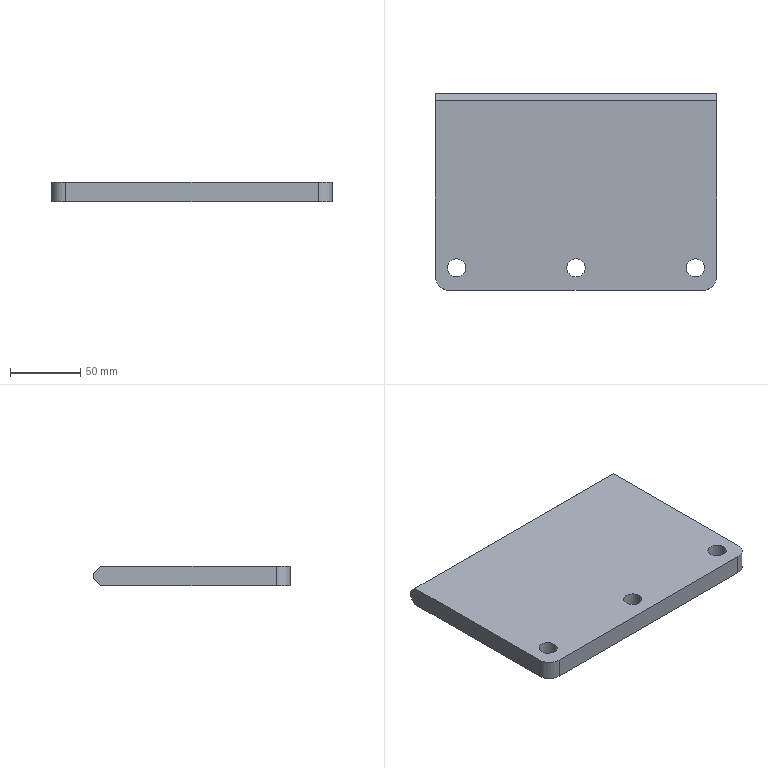Part | SolidWorks | features ICE 2, Chamfer 1, Extrusion 1, Fillet 1 | 1 solid | 16 faces | box 200 x 140 x 14 mm | volume 380824 mm3 | cylinder 8 | plane 8 | commonest cylinder face diameters 13 x6 20 x2
STEP:
#1=CARTESIAN_POINT('',(191.5,16.,14.));
#2=VERTEX_POINT('',#1);
#3=CARTESIAN_POINT('',(178.5,16.,14.));
#4=VERTEX_POINT('',#3);
#5=CARTESIAN_POINT('',(185.,16.,14.));
#6=DIRECTION('',(0.,0.,-1.));
#7=DIRECTION('',(-1.,0.,0.));
#8=AXIS2_PLACEMENT_3D('',#5,#6,#7);
#9=CIRCLE('',#8,6.5);
#10=EDGE_CURVE('',#2,#4,#9,.T.);
#11=ORIENTED_EDGE('',*,*,#10,.F.);
#12=CARTESIAN_POINT('',(191.5,16.,0.));
#13=VERTEX_POINT('',#12);
#14=CARTESIAN_POINT('',(191.5,16.,14.));
#15=DIRECTION('',(0.,0.,-1.));
#16=VECTOR('',#15,1000.);
#17=LINE('',#14,#16);
#18=EDGE_CURVE('',#2,#13,#17,.T.);
#19=ORIENTED_EDGE('',*,*,#18,.T.);
#20=CARTESIAN_POINT('',(178.5,16.,0.));
#21=VERTEX_POINT('',#20);
#22=CARTESIAN_POINT('',(185.,16.,0.));
#23=DIRECTION('',(0.,0.,-1.));
#24=DIRECTION('',(-1.,0.,0.));
#25=AXIS2_PLACEMENT_3D('',#22,#23,#24);
#26=CIRCLE('',#25,6.5);
#27=EDGE_CURVE('',#13,#21,#26,.T.);
#28=ORIENTED_EDGE('',*,*,#27,.T.);
#29=CARTESIAN_POINT('',(178.5,16.,14.));
#30=DIRECTION('',(0.,0.,-1.));
#31=VECTOR('',#30,1000.);
#32=LINE('',#29,#31);
#33=EDGE_CURVE('',#4,#21,#32,.T.);
#34=ORIENTED_EDGE('',*,*,#33,.F.);
#35=EDGE_LOOP('',(#11,#19,#28,#34));
#36=FACE_OUTER_BOUND('',#35,.T.);
#37=CARTESIAN_POINT('',(185.,16.,14.));
#38=DIRECTION('',(0.,0.,-1.));
#39=DIRECTION('',(-1.,0.,0.));
#40=AXIS2_PLACEMENT_3D('',#37,#38,#39);
#41=CYLINDRICAL_SURFACE('',#40,6.5);
#42=ADVANCED_FACE('',(#36),#41,.F.);
#43=CARTESIAN_POINT('',(106.5,16.,14.));
#44=VERTEX_POINT('',#43);
#45=CARTESIAN_POINT('',(93.5,16.,14.));
#46=VERTEX_POINT('',#45);
#47=CARTESIAN_POINT('',(100.,16.,14.));
#48=DIRECTION('',(0.,0.,-1.));
#49=DIRECTION('',(-1.,0.,0.));
#50=AXIS2_PLACEMENT_3D('',#47,#48,#49);
#51=CIRCLE('',#50,6.5);
#52=EDGE_CURVE('',#44,#46,#51,.T.);
#53=ORIENTED_EDGE('',*,*,#52,.F.);
#54=CARTESIAN_POINT('',(106.5,16.,0.));
#55=VERTEX_POINT('',#54);
#56=CARTESIAN_POINT('',(106.5,16.,14.));
#57=DIRECTION('',(0.,0.,-1.));
#58=VECTOR('',#57,1000.);
#59=LINE('',#56,#58);
#60=EDGE_CURVE('',#44,#55,#59,.T.);
#61=ORIENTED_EDGE('',*,*,#60,.T.);
#62=CARTESIAN_POINT('',(93.5,16.,0.));
#63=VERTEX_POINT('',#62);
#64=CARTESIAN_POINT('',(100.,16.,0.));
#65=DIRECTION('',(0.,0.,-1.));
#66=DIRECTION('',(-1.,0.,0.));
#67=AXIS2_PLACEMENT_3D('',#64,#65,#66);
#68=CIRCLE('',#67,6.5);
#69=EDGE_CURVE('',#55,#63,#68,.T.);
#70=ORIENTED_EDGE('',*,*,#69,.T.);
#71=CARTESIAN_POINT('',(93.5,16.,14.));
#72=DIRECTION('',(0.,0.,-1.));
#73=VECTOR('',#72,1000.);
#74=LINE('',#71,#73);
#75=EDGE_CURVE('',#46,#63,#74,.T.);
#76=ORIENTED_EDGE('',*,*,#75,.F.);
#77=EDGE_LOOP('',(#53,#61,#70,#76));
#78=FACE_OUTER_BOUND('',#77,.T.);
#79=CARTESIAN_POINT('',(100.,16.,14.));
#80=DIRECTION('',(0.,0.,-1.));
#81=DIRECTION('',(-1.,0.,0.));
#82=AXIS2_PLACEMENT_3D('',#79,#80,#81);
#83=CYLINDRICAL_SURFACE('',#82,6.5);
#84=ADVANCED_FACE('',(#78),#83,.F.);
#85=CARTESIAN_POINT('',(21.5,16.,14.));
#86=VERTEX_POINT('',#85);
#87=CARTESIAN_POINT('',(8.5,16.,14.));
#88=VERTEX_POINT('',#87);
#89=CARTESIAN_POINT('',(15.,16.,14.));
#90=DIRECTION('',(0.,0.,-1.));
#91=DIRECTION('',(-1.,0.,0.));
#92=AXIS2_PLACEMENT_3D('',#89,#90,#91);
#93=CIRCLE('',#92,6.5);
#94=EDGE_CURVE('',#86,#88,#93,.T.);
#95=ORIENTED_EDGE('',*,*,#94,.F.);
#96=CARTESIAN_POINT('',(21.5,16.,0.));
#97=VERTEX_POINT('',#96);
#98=CARTESIAN_POINT('',(21.5,16.,14.));
#99=DIRECTION('',(0.,0.,-1.));
#100=VECTOR('',#99,1000.);
#101=LINE('',#98,#100);
#102=EDGE_CURVE('',#86,#97,#101,.T.);
#103=ORIENTED_EDGE('',*,*,#102,.T.);
#104=CARTESIAN_POINT('',(8.5,16.,0.));
#105=VERTEX_POINT('',#104);
#106=CARTESIAN_POINT('',(15.,16.,0.));
#107=DIRECTION('',(0.,0.,-1.));
#108=DIRECTION('',(-1.,0.,0.));
#109=AXIS2_PLACEMENT_3D('',#106,#107,#108);
#110=CIRCLE('',#109,6.5);
#111=EDGE_CURVE('',#97,#105,#110,.T.);
#112=ORIENTED_EDGE('',*,*,#111,.T.);
#113=CARTESIAN_POINT('',(8.5,16.,14.));
#114=DIRECTION('',(0.,0.,-1.));
#115=VECTOR('',#114,1000.);
#116=LINE('',#113,#115);
#117=EDGE_CURVE('',#88,#105,#116,.T.);
#118=ORIENTED_EDGE('',*,*,#117,.F.);
#119=EDGE_LOOP('',(#95,#103,#112,#118));
#120=FACE_OUTER_BOUND('',#119,.T.);
#121=CARTESIAN_POINT('',(15.,16.,14.));
#122=DIRECTION('',(0.,0.,-1.));
#123=DIRECTION('',(-1.,0.,0.));
#124=AXIS2_PLACEMENT_3D('',#121,#122,#123);
#125=CYLINDRICAL_SURFACE('',#124,6.5);
#126=ADVANCED_FACE('',(#120),#125,.F.);
#127=CARTESIAN_POINT('',(0.,135.,0.));
#128=VERTEX_POINT('',#127);
#129=CARTESIAN_POINT('',(0.,10.,0.));
#130=VERTEX_POINT('',#129);
#131=CARTESIAN_POINT('',(0.,0.,0.));
#132=DIRECTION('',(0.,-1.,0.));
#133=VECTOR('',#132,1000.);
#134=LINE('',#131,#133);
#135=EDGE_CURVE('',#128,#130,#134,.T.);
#136=ORIENTED_EDGE('',*,*,#135,.T.);
#137=CARTESIAN_POINT('',(0.,10.,14.));
#138=VERTEX_POINT('',#137);
#139=CARTESIAN_POINT('',(0.,10.,14.));
#140=DIRECTION('',(0.,0.,1.));
#141=VECTOR('',#140,1000.);
#142=LINE('',#139,#141);
#143=EDGE_CURVE('',#130,#138,#142,.T.);
#144=ORIENTED_EDGE('',*,*,#143,.T.);
#145=CARTESIAN_POINT('',(0.,135.,14.));
#146=VERTEX_POINT('',#145);
#147=CARTESIAN_POINT('',(0.,0.,14.));
#148=DIRECTION('',(0.,-1.,0.));
#149=VECTOR('',#148,1000.);
#150=LINE('',#147,#149);
#151=EDGE_CURVE('',#146,#138,#150,.T.);
#152=ORIENTED_EDGE('',*,*,#151,.F.);
#153=CARTESIAN_POINT('',(0.,140.,9.));
#154=VERTEX_POINT('',#153);
#155=CARTESIAN_POINT('',(0.,135.,14.));
#156=DIRECTION('',(0.,0.7071,-0.7071));
#157=VECTOR('',#156,1000.);
#158=LINE('',#155,#157);
#159=EDGE_CURVE('',#146,#154,#158,.T.);
#160=ORIENTED_EDGE('',*,*,#159,.T.);
#161=CARTESIAN_POINT('',(0.,140.,5.));
#162=VERTEX_POINT('',#161);
#163=CARTESIAN_POINT('',(0.,140.,14.));
#164=DIRECTION('',(0.,0.,-1.));
#165=VECTOR('',#164,1000.);
#166=LINE('',#163,#165);
#167=EDGE_CURVE('',#154,#162,#166,.T.);
#168=ORIENTED_EDGE('',*,*,#167,.T.);
#169=CARTESIAN_POINT('',(0.,140.,5.));
#170=DIRECTION('',(0.,-0.7071,-0.7071));
#171=VECTOR('',#170,1000.);
#172=LINE('',#169,#171);
#173=EDGE_CURVE('',#162,#128,#172,.T.);
#174=ORIENTED_EDGE('',*,*,#173,.T.);
#175=EDGE_LOOP('',(#136,#144,#152,#160,#168,#174));
#176=FACE_OUTER_BOUND('',#175,.T.);
#177=CARTESIAN_POINT('',(0.,0.,14.));
#178=DIRECTION('',(1.,0.,0.));
#179=DIRECTION('',(0.,0.,-1.));
#180=AXIS2_PLACEMENT_3D('',#177,#178,#179);
#181=PLANE('',#180);
#182=ADVANCED_FACE('',(#176),#181,.F.);
#183=CARTESIAN_POINT('',(10.,0.,0.));
#184=VERTEX_POINT('',#183);
#185=CARTESIAN_POINT('',(190.,0.,0.));
#186=VERTEX_POINT('',#185);
#187=CARTESIAN_POINT('',(0.,0.,0.));
#188=DIRECTION('',(1.,0.,0.));
#189=VECTOR('',#188,1000.);
#190=LINE('',#187,#189);
#191=EDGE_CURVE('',#184,#186,#190,.T.);
#192=ORIENTED_EDGE('',*,*,#191,.T.);
#193=CARTESIAN_POINT('',(190.,0.,14.));
#194=VERTEX_POINT('',#193);
#195=CARTESIAN_POINT('',(190.,0.,14.));
#196=DIRECTION('',(0.,0.,1.));
#197=VECTOR('',#196,1000.);
#198=LINE('',#195,#197);
#199=EDGE_CURVE('',#186,#194,#198,.T.);
#200=ORIENTED_EDGE('',*,*,#199,.T.);
#201=CARTESIAN_POINT('',(10.,0.,14.));
#202=VERTEX_POINT('',#201);
#203=CARTESIAN_POINT('',(0.,0.,14.));
#204=DIRECTION('',(1.,0.,0.));
#205=VECTOR('',#204,1000.);
#206=LINE('',#203,#205);
#207=EDGE_CURVE('',#202,#194,#206,.T.);
#208=ORIENTED_EDGE('',*,*,#207,.F.);
#209=CARTESIAN_POINT('',(10.,0.,14.));
#210=DIRECTION('',(0.,0.,-1.));
#211=VECTOR('',#210,1000.);
#212=LINE('',#209,#211);
#213=EDGE_CURVE('',#202,#184,#212,.T.);
#214=ORIENTED_EDGE('',*,*,#213,.T.);
#215=EDGE_LOOP('',(#192,#200,#208,#214));
#216=FACE_OUTER_BOUND('',#215,.T.);
#217=CARTESIAN_POINT('',(0.,0.,14.));
#218=DIRECTION('',(0.,1.,0.));
#219=DIRECTION('',(0.,0.,1.));
#220=AXIS2_PLACEMENT_3D('',#217,#218,#219);
#221=PLANE('',#220);
#222=ADVANCED_FACE('',(#216),#221,.F.);
#223=CARTESIAN_POINT('',(200.,10.,14.));
#224=VERTEX_POINT('',#223);
#225=CARTESIAN_POINT('',(200.,135.,14.));
#226=VERTEX_POINT('',#225);
#227=CARTESIAN_POINT('',(200.,0.,14.));
#228=DIRECTION('',(0.,1.,0.));
#229=VECTOR('',#228,1000.);
#230=LINE('',#227,#229);
#231=EDGE_CURVE('',#224,#226,#230,.T.);
#232=ORIENTED_EDGE('',*,*,#231,.F.);
#233=CARTESIAN_POINT('',(200.,10.,0.));
#234=VERTEX_POINT('',#233);
#235=CARTESIAN_POINT('',(200.,10.,14.));
#236=DIRECTION('',(0.,0.,-1.));
#237=VECTOR('',#236,1000.);
#238=LINE('',#235,#237);
#239=EDGE_CURVE('',#224,#234,#238,.T.);
#240=ORIENTED_EDGE('',*,*,#239,.T.);
#241=CARTESIAN_POINT('',(200.,135.,0.));
#242=VERTEX_POINT('',#241);
#243=CARTESIAN_POINT('',(200.,0.,0.));
#244=DIRECTION('',(0.,1.,0.));
#245=VECTOR('',#244,1000.);
#246=LINE('',#243,#245);
#247=EDGE_CURVE('',#234,#242,#246,.T.);
#248=ORIENTED_EDGE('',*,*,#247,.T.);
#249=CARTESIAN_POINT('',(200.,140.,5.));
#250=VERTEX_POINT('',#249);
#251=CARTESIAN_POINT('',(200.,140.,5.));
#252=DIRECTION('',(0.,0.7071,0.7071));
#253=VECTOR('',#252,1000.);
#254=LINE('',#251,#253);
#255=EDGE_CURVE('',#242,#250,#254,.T.);
#256=ORIENTED_EDGE('',*,*,#255,.T.);
#257=CARTESIAN_POINT('',(200.,140.,9.));
#258=VERTEX_POINT('',#257);
#259=CARTESIAN_POINT('',(200.,140.,14.));
#260=DIRECTION('',(0.,0.,-1.));
#261=VECTOR('',#260,1000.);
#262=LINE('',#259,#261);
#263=EDGE_CURVE('',#258,#250,#262,.T.);
#264=ORIENTED_EDGE('',*,*,#263,.F.);
#265=CARTESIAN_POINT('',(200.,135.,14.));
#266=DIRECTION('',(0.,-0.7071,0.7071));
#267=VECTOR('',#266,1000.);
#268=LINE('',#265,#267);
#269=EDGE_CURVE('',#258,#226,#268,.T.);
#270=ORIENTED_EDGE('',*,*,#269,.T.);
#271=EDGE_LOOP('',(#232,#240,#248,#256,#264,#270));
#272=FACE_OUTER_BOUND('',#271,.T.);
#273=CARTESIAN_POINT('',(200.,0.,14.));
#274=DIRECTION('',(-1.,0.,0.));
#275=DIRECTION('',(0.,0.,1.));
#276=AXIS2_PLACEMENT_3D('',#273,#274,#275);
#277=PLANE('',#276);
#278=ADVANCED_FACE('',(#272),#277,.F.);
#279=ORIENTED_EDGE('',*,*,#167,.F.);
#280=CARTESIAN_POINT('',(0.,140.,9.));
#281=DIRECTION('',(1.,0.,0.));
#282=VECTOR('',#281,1000.);
#283=LINE('',#280,#282);
#284=EDGE_CURVE('',#154,#258,#283,.T.);
#285=ORIENTED_EDGE('',*,*,#284,.T.);
#286=ORIENTED_EDGE('',*,*,#263,.T.);
#287=CARTESIAN_POINT('',(0.,140.,5.));
#288=DIRECTION('',(-1.,0.,0.));
#289=VECTOR('',#288,1000.);
#290=LINE('',#287,#289);
#291=EDGE_CURVE('',#250,#162,#290,.T.);
#292=ORIENTED_EDGE('',*,*,#291,.T.);
#293=EDGE_LOOP('',(#279,#285,#286,#292));
#294=FACE_OUTER_BOUND('',#293,.T.);
#295=CARTESIAN_POINT('',(0.,140.,14.));
#296=DIRECTION('',(0.,-1.,0.));
#297=DIRECTION('',(0.,0.,-1.));
#298=AXIS2_PLACEMENT_3D('',#295,#296,#297);
#299=PLANE('',#298);
#300=ADVANCED_FACE('',(#294),#299,.F.);
#301=CARTESIAN_POINT('',(185.,16.,14.));
#302=DIRECTION('',(0.,0.,-1.));
#303=DIRECTION('',(-1.,0.,0.));
#304=AXIS2_PLACEMENT_3D('',#301,#302,#303);
#305=CIRCLE('',#304,6.5);
#306=EDGE_CURVE('',#4,#2,#305,.T.);
#307=ORIENTED_EDGE('',*,*,#306,.T.);
#308=ORIENTED_EDGE('',*,*,#10,.T.);
#309=EDGE_LOOP('',(#307,#308));
#310=FACE_BOUND('',#309,.T.);
#311=CARTESIAN_POINT('',(100.,16.,14.));
#312=DIRECTION('',(0.,0.,-1.));
#313=DIRECTION('',(-1.,0.,0.));
#314=AXIS2_PLACEMENT_3D('',#311,#312,#313);
#315=CIRCLE('',#314,6.5);
#316=EDGE_CURVE('',#46,#44,#315,.T.);
#317=ORIENTED_EDGE('',*,*,#316,.T.);
#318=ORIENTED_EDGE('',*,*,#52,.T.);
#319=EDGE_LOOP('',(#317,#318));
#320=FACE_BOUND('',#319,.T.);
#321=CARTESIAN_POINT('',(15.,16.,14.));
#322=DIRECTION('',(0.,0.,-1.));
#323=DIRECTION('',(-1.,0.,0.));
#324=AXIS2_PLACEMENT_3D('',#321,#322,#323);
#325=CIRCLE('',#324,6.5);
#326=EDGE_CURVE('',#88,#86,#325,.T.);
#327=ORIENTED_EDGE('',*,*,#326,.T.);
#328=ORIENTED_EDGE('',*,*,#94,.T.);
#329=EDGE_LOOP('',(#327,#328));
#330=FACE_BOUND('',#329,.T.);
#331=ORIENTED_EDGE('',*,*,#207,.T.);
#332=CARTESIAN_POINT('',(190.,10.,14.));
#333=DIRECTION('',(0.,0.,1.));
#334=DIRECTION('',(-1.,0.,0.));
#335=AXIS2_PLACEMENT_3D('',#332,#333,#334);
#336=CIRCLE('',#335,10.);
#337=EDGE_CURVE('',#194,#224,#336,.T.);
#338=ORIENTED_EDGE('',*,*,#337,.T.);
#339=ORIENTED_EDGE('',*,*,#231,.T.);
#340=CARTESIAN_POINT('',(0.,135.,14.));
#341=DIRECTION('',(-1.,0.,0.));
#342=VECTOR('',#341,1000.);
#343=LINE('',#340,#342);
#344=EDGE_CURVE('',#226,#146,#343,.T.);
#345=ORIENTED_EDGE('',*,*,#344,.T.);
#346=ORIENTED_EDGE('',*,*,#151,.T.);
#347=CARTESIAN_POINT('',(10.,10.,14.));
#348=DIRECTION('',(0.,0.,1.));
#349=DIRECTION('',(-1.,0.,0.));
#350=AXIS2_PLACEMENT_3D('',#347,#348,#349);
#351=CIRCLE('',#350,10.);
#352=EDGE_CURVE('',#138,#202,#351,.T.);
#353=ORIENTED_EDGE('',*,*,#352,.T.);
#354=EDGE_LOOP('',(#331,#338,#339,#345,#346,#353));
#355=FACE_OUTER_BOUND('',#354,.T.);
#356=CARTESIAN_POINT('',(0.,0.,14.));
#357=DIRECTION('',(0.,0.,-1.));
#358=DIRECTION('',(-1.,0.,0.));
#359=AXIS2_PLACEMENT_3D('',#356,#357,#358);
#360=PLANE('',#359);
#361=ADVANCED_FACE('',(#310,#320,#330,#355),#360,.F.);
#362=CARTESIAN_POINT('',(185.,16.,0.));
#363=DIRECTION('',(0.,0.,-1.));
#364=DIRECTION('',(-1.,0.,0.));
#365=AXIS2_PLACEMENT_3D('',#362,#363,#364);
#366=CIRCLE('',#365,6.5);
#367=EDGE_CURVE('',#21,#13,#366,.T.);
#368=ORIENTED_EDGE('',*,*,#367,.F.);
#369=ORIENTED_EDGE('',*,*,#27,.F.);
#370=EDGE_LOOP('',(#368,#369));
#371=FACE_BOUND('',#370,.T.);
#372=CARTESIAN_POINT('',(100.,16.,0.));
#373=DIRECTION('',(0.,0.,-1.));
#374=DIRECTION('',(-1.,0.,0.));
#375=AXIS2_PLACEMENT_3D('',#372,#373,#374);
#376=CIRCLE('',#375,6.5);
#377=EDGE_CURVE('',#63,#55,#376,.T.);
#378=ORIENTED_EDGE('',*,*,#377,.F.);
#379=ORIENTED_EDGE('',*,*,#69,.F.);
#380=EDGE_LOOP('',(#378,#379));
#381=FACE_BOUND('',#380,.T.);
#382=CARTESIAN_POINT('',(15.,16.,0.));
#383=DIRECTION('',(0.,0.,-1.));
#384=DIRECTION('',(-1.,0.,0.));
#385=AXIS2_PLACEMENT_3D('',#382,#383,#384);
#386=CIRCLE('',#385,6.5);
#387=EDGE_CURVE('',#105,#97,#386,.T.);
#388=ORIENTED_EDGE('',*,*,#387,.F.);
#389=ORIENTED_EDGE('',*,*,#111,.F.);
#390=EDGE_LOOP('',(#388,#389));
#391=FACE_BOUND('',#390,.T.);
#392=ORIENTED_EDGE('',*,*,#247,.F.);
#393=CARTESIAN_POINT('',(190.,10.,0.));
#394=DIRECTION('',(0.,0.,-1.));
#395=DIRECTION('',(-1.,0.,0.));
#396=AXIS2_PLACEMENT_3D('',#393,#394,#395);
#397=CIRCLE('',#396,10.);
#398=EDGE_CURVE('',#234,#186,#397,.T.);
#399=ORIENTED_EDGE('',*,*,#398,.T.);
#400=ORIENTED_EDGE('',*,*,#191,.F.);
#401=CARTESIAN_POINT('',(10.,10.,0.));
#402=DIRECTION('',(0.,0.,-1.));
#403=DIRECTION('',(-1.,0.,0.));
#404=AXIS2_PLACEMENT_3D('',#401,#402,#403);
#405=CIRCLE('',#404,10.);
#406=EDGE_CURVE('',#184,#130,#405,.T.);
#407=ORIENTED_EDGE('',*,*,#406,.T.);
#408=ORIENTED_EDGE('',*,*,#135,.F.);
#409=CARTESIAN_POINT('',(200.,135.,0.));
#410=DIRECTION('',(1.,0.,0.));
#411=VECTOR('',#410,1000.);
#412=LINE('',#409,#411);
#413=EDGE_CURVE('',#128,#242,#412,.T.);
#414=ORIENTED_EDGE('',*,*,#413,.T.);
#415=EDGE_LOOP('',(#392,#399,#400,#407,#408,#414));
#416=FACE_OUTER_BOUND('',#415,.T.);
#417=CARTESIAN_POINT('',(0.,0.,0.));
#418=DIRECTION('',(0.,0.,-1.));
#419=DIRECTION('',(-1.,0.,0.));
#420=AXIS2_PLACEMENT_3D('',#417,#418,#419);
#421=PLANE('',#420);
#422=ADVANCED_FACE('',(#371,#381,#391,#416),#421,.T.);
#423=ORIENTED_EDGE('',*,*,#269,.F.);
#424=ORIENTED_EDGE('',*,*,#284,.F.);
#425=ORIENTED_EDGE('',*,*,#159,.F.);
#426=ORIENTED_EDGE('',*,*,#344,.F.);
#427=EDGE_LOOP('',(#423,#424,#425,#426));
#428=FACE_OUTER_BOUND('',#427,.T.);
#429=CARTESIAN_POINT('',(0.,135.,14.));
#430=DIRECTION('',(0.,-0.7071,-0.7071));
#431=DIRECTION('',(-1.,0.,0.));
#432=AXIS2_PLACEMENT_3D('',#429,#430,#431);
#433=PLANE('',#432);
#434=ADVANCED_FACE('',(#428),#433,.F.);
#435=ORIENTED_EDGE('',*,*,#255,.F.);
#436=ORIENTED_EDGE('',*,*,#413,.F.);
#437=ORIENTED_EDGE('',*,*,#173,.F.);
#438=ORIENTED_EDGE('',*,*,#291,.F.);
#439=EDGE_LOOP('',(#435,#436,#437,#438));
#440=FACE_OUTER_BOUND('',#439,.T.);
#441=CARTESIAN_POINT('',(0.,140.,5.));
#442=DIRECTION('',(0.,0.7071,-0.7071));
#443=DIRECTION('',(1.,0.,0.));
#444=AXIS2_PLACEMENT_3D('',#441,#442,#443);
#445=PLANE('',#444);
#446=ADVANCED_FACE('',(#440),#445,.T.);
#447=ORIENTED_EDGE('',*,*,#102,.F.);
#448=ORIENTED_EDGE('',*,*,#326,.F.);
#449=ORIENTED_EDGE('',*,*,#117,.T.);
#450=ORIENTED_EDGE('',*,*,#387,.T.);
#451=EDGE_LOOP('',(#447,#448,#449,#450));
#452=FACE_OUTER_BOUND('',#451,.T.);
#453=CARTESIAN_POINT('',(15.,16.,14.));
#454=DIRECTION('',(0.,0.,-1.));
#455=DIRECTION('',(-1.,0.,0.));
#456=AXIS2_PLACEMENT_3D('',#453,#454,#455);
#457=CYLINDRICAL_SURFACE('',#456,6.5);
#458=ADVANCED_FACE('',(#452),#457,.F.);
#459=ORIENTED_EDGE('',*,*,#60,.F.);
#460=ORIENTED_EDGE('',*,*,#316,.F.);
#461=ORIENTED_EDGE('',*,*,#75,.T.);
#462=ORIENTED_EDGE('',*,*,#377,.T.);
#463=EDGE_LOOP('',(#459,#460,#461,#462));
#464=FACE_OUTER_BOUND('',#463,.T.);
#465=CARTESIAN_POINT('',(100.,16.,14.));
#466=DIRECTION('',(0.,0.,-1.));
#467=DIRECTION('',(-1.,0.,0.));
#468=AXIS2_PLACEMENT_3D('',#465,#466,#467);
#469=CYLINDRICAL_SURFACE('',#468,6.5);
#470=ADVANCED_FACE('',(#464),#469,.F.);
#471=ORIENTED_EDGE('',*,*,#18,.F.);
#472=ORIENTED_EDGE('',*,*,#306,.F.);
#473=ORIENTED_EDGE('',*,*,#33,.T.);
#474=ORIENTED_EDGE('',*,*,#367,.T.);
#475=EDGE_LOOP('',(#471,#472,#473,#474));
#476=FACE_OUTER_BOUND('',#475,.T.);
#477=CARTESIAN_POINT('',(185.,16.,14.));
#478=DIRECTION('',(0.,0.,-1.));
#479=DIRECTION('',(-1.,0.,0.));
#480=AXIS2_PLACEMENT_3D('',#477,#478,#479);
#481=CYLINDRICAL_SURFACE('',#480,6.5);
#482=ADVANCED_FACE('',(#476),#481,.F.);
#483=ORIENTED_EDGE('',*,*,#337,.F.);
#484=ORIENTED_EDGE('',*,*,#199,.F.);
#485=ORIENTED_EDGE('',*,*,#398,.F.);
#486=ORIENTED_EDGE('',*,*,#239,.F.);
#487=EDGE_LOOP('',(#483,#484,#485,#486));
#488=FACE_OUTER_BOUND('',#487,.T.);
#489=CARTESIAN_POINT('',(190.,10.,14.));
#490=DIRECTION('',(0.,0.,-1.));
#491=DIRECTION('',(-1.,0.,0.));
#492=AXIS2_PLACEMENT_3D('',#489,#490,#491);
#493=CYLINDRICAL_SURFACE('',#492,10.);
#494=ADVANCED_FACE('',(#488),#493,.T.);
#495=ORIENTED_EDGE('',*,*,#352,.F.);
#496=ORIENTED_EDGE('',*,*,#143,.F.);
#497=ORIENTED_EDGE('',*,*,#406,.F.);
#498=ORIENTED_EDGE('',*,*,#213,.F.);
#499=EDGE_LOOP('',(#495,#496,#497,#498));
#500=FACE_OUTER_BOUND('',#499,.T.);
#501=CARTESIAN_POINT('',(10.,10.,14.));
#502=DIRECTION('',(0.,0.,-1.));
#503=DIRECTION('',(-1.,0.,0.));
#504=AXIS2_PLACEMENT_3D('',#501,#502,#503);
#505=CYLINDRICAL_SURFACE('',#504,10.);
#506=ADVANCED_FACE('',(#500),#505,.T.);
#507=CLOSED_SHELL('',(#42,#84,#126,#182,#222,#278,#300,#361,#422,#434,#446,#458,#470,#482,#494,#506));
#508=MANIFOLD_SOLID_BREP('',#507);
#509=CARTESIAN_POINT('',(0.,0.,0.));
#510=DIRECTION('',(0.,0.,1.));
#511=DIRECTION('',(1.,0.,0.));
#512=AXIS2_PLACEMENT_3D('',#509,#510,#511);
#513=(LENGTH_UNIT()NAMED_UNIT(*)SI_UNIT(.MILLI.,.METRE.));
#514=UNCERTAINTY_MEASURE_WITH_UNIT(LENGTH_MEASURE(0.00001),#513,'','');
#515=(NAMED_UNIT(*)PLANE_ANGLE_UNIT()SI_UNIT($,.RADIAN.));
#516=(NAMED_UNIT(*)SI_UNIT($,.STERADIAN.)SOLID_ANGLE_UNIT());
#517=(GEOMETRIC_REPRESENTATION_CONTEXT(3)GLOBAL_UNCERTAINTY_ASSIGNED_CONTEXT((#514))GLOBAL_UNIT_ASSIGNED_CONTEXT((#513,#515,#516))REPRESENTATION_CONTEXT('',''));
#518=ADVANCED_BREP_SHAPE_REPRESENTATION('',(#508,#512),#517);